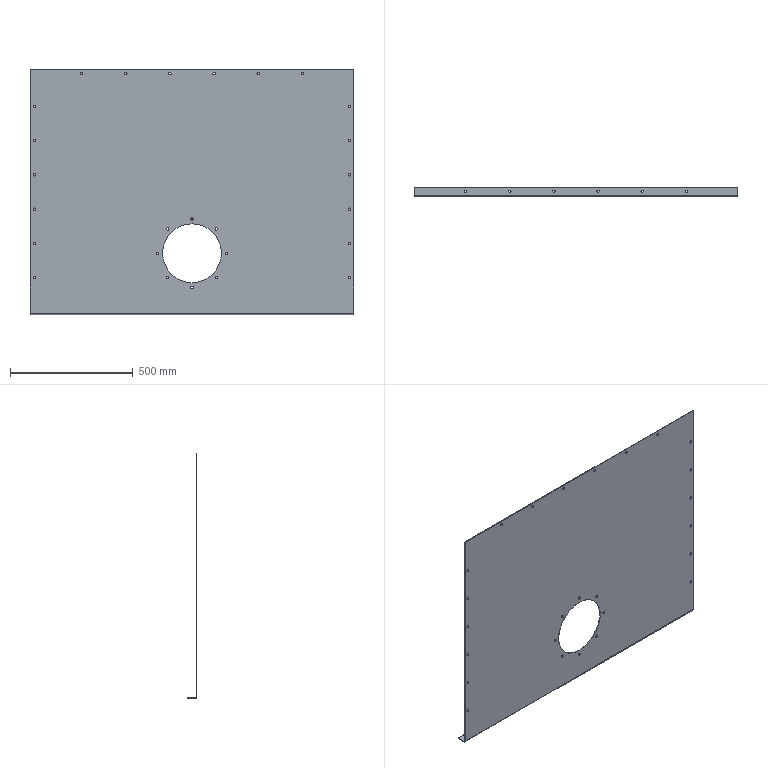Part | SolidWorks | features ICE 3, CirPattern 1, EdgeFlange 1, FlatPattern 1, RefAxis 1, SMBaseFlange 1, SheetMetal 1 | 1 solid | 80 faces | box 1320 x 40 x 1000 mm | volume 3955615 mm3 | cylinder 68 | plane 12 | commonest cylinder face diameters 10 x64 240 x2 6 x1 12 x1